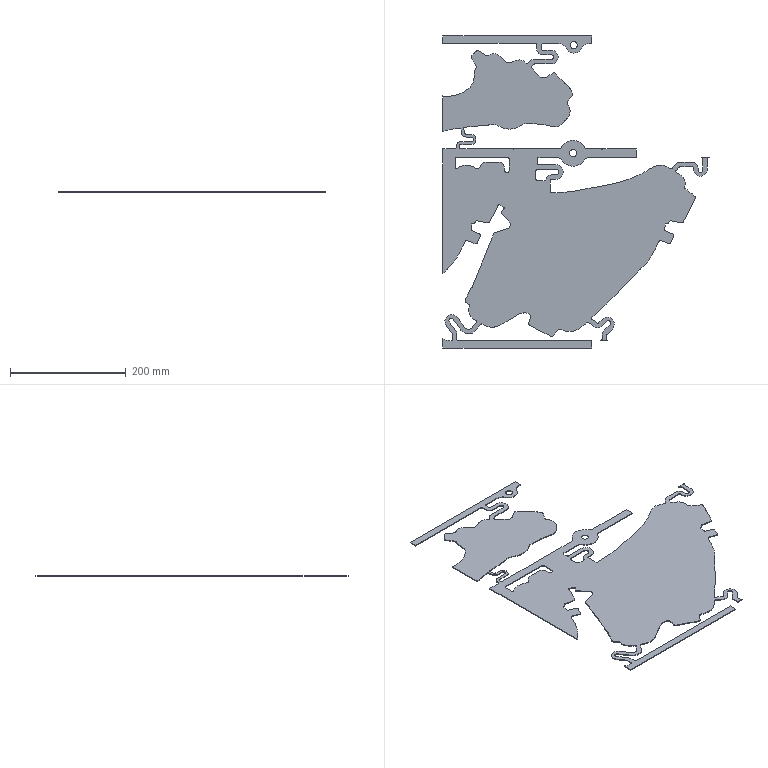Part | STEP file | gslz 2016.10.28-13_id222_x_t | 1 solid | 381 faces | box 460.712 x 540 x 1.25 mm | volume 153991 mm3 | plane 198 | cylinder 183 | commonest cylinder face diameters 4 x58 6 x25 10 x11 20 x11 8 x10 30 x8